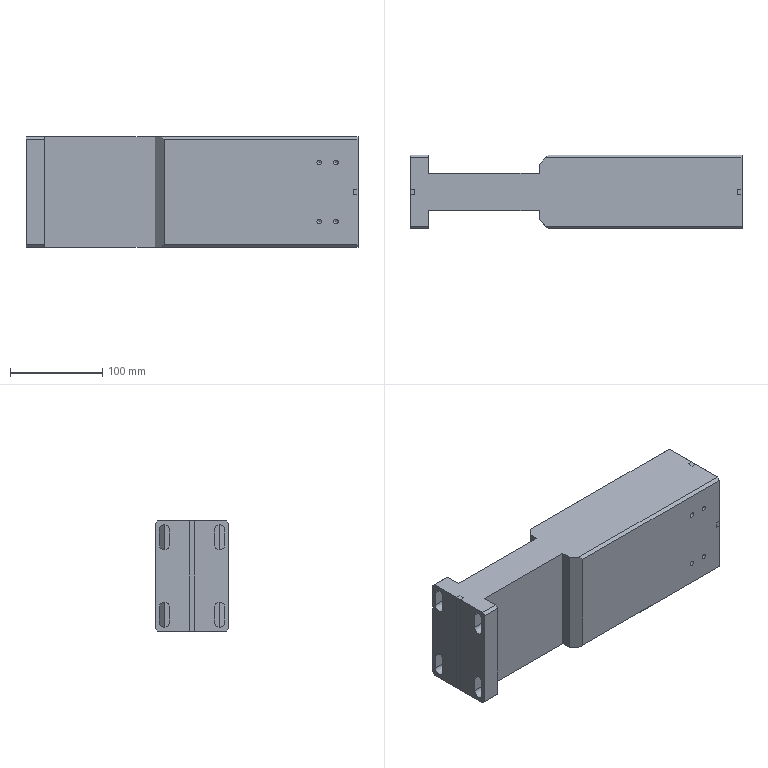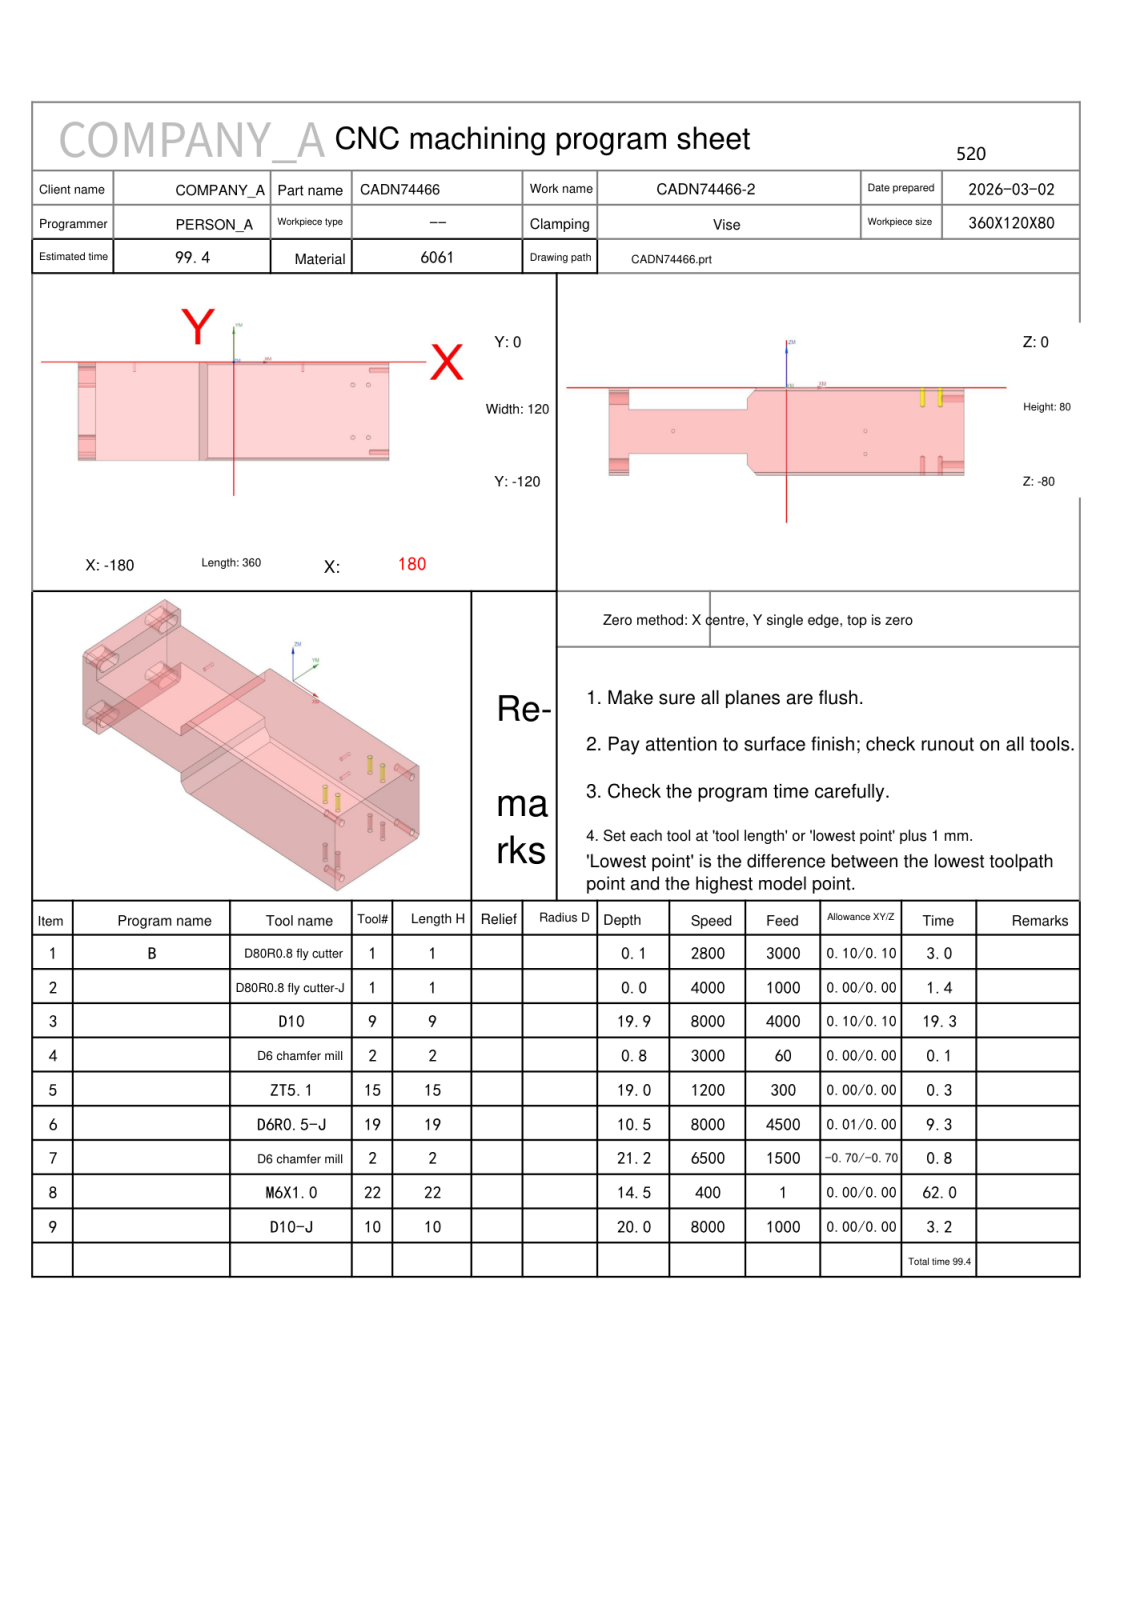NC program | NX | posted by the shop | part box 360 x 80 x 120 mm
Lines 4234 to 6245 of 6245:
N4 T02 M06
(D6 chamfer mill  D=6. R=0. H=02 ce=0.00 di=0.10)
G00 G90 G54 X138. Y-92. M03 S3000
G43 H02 Z50.
M08
G98 G81 X138. Y-92. Z-.8 R1. F60.
X156.
Y-28.
X138.
G80
G00 Z50.
G91 G28 Z0.0
M05
M09
G91 G28 Z0.0
M01
N5 T15 M06
(ZT5.1 D=5.1 DR_a=118 H=15)
G00 G90 G54 X138. Y-92. M03 S1200
G43 H15 Z50.
M08
G98 G83 X138. Y-92. Z-19. R1. F300. Q1.
X156.
Y-28.
X138.
G80
G00 Z50.
G91 G28 Z0.0
M05
M09
G91 G28 Z0.0
M01
N6 T19 M06
(D6R0.5-J  D=6. R=0.5 H=19 ce=0.01 di=0.00)
G00 G90 G54 X-32.786 Y-123.359 M03 S8000
G43 H19 Z14.5
M08
Z.429
G01 Z-.071 F4500.
Y-118.232
Y-1.768
X-32.857 Y-1.697 Z-.141
Y-118.303
X-32.927 Y-118.375 Z-.212
X-32.929 Y-118.275
Y-1.725
X-32.927 Y-1.625
X-32.996 Y-1.554 Z-.283
X-33. Y-1.725
Y-118.275
X-32.996 Y-118.446
X-33.068 Y-118.517 Z-.354
X-33.071 Y-118.275
Y-1.725
X-33.068 Y-1.483
X-33.14 Y-1.412 Z-.424
X-33.141 Y-2.722
Y-117.278
X-33.14 Y-118.588
X-33.21 Y-118.66 Z-.495
X-33.212 Y-118.622
Y-1.378
X-33.21 Y-1.34
X-33.28 Y-1.269 Z-.566
X-33.283 Y-1.378
Y-118.622
X-33.28 Y-118.731
X-33.35 Y-118.802 Z-.636
X-33.354 Y-118.622
Y-1.378
X-33.35 Y-1.198
X-33.421 Y-1.127 Z-.707
X-33.424 Y-1.378
Y-118.622
X-33.421 Y-118.873
X-33.494 Y-118.944 Z-.778
X-33.495 Y-117.631
Y-2.369
X-33.494 Y-1.056
X-33.563 Y-.985 Z-.849
X-33.566 Y-1.031
Y-118.969
X-33.563 Y-119.015
X-33.633 Y-119.085 Z-.919
X-33.636 Y-118.969
Y-1.031
X-33.633 Y-.915
X-33.704 Y-.844 Z-.99
X-33.707 Y-1.031
Y-118.969
X-33.704 Y-119.156
X-33.775 Y-119.227 Z-1.061
X-33.778 Y-118.969
Y-1.031
X-33.775 Y-.773
X-33.848 Y-.703 Z-1.131
Y-2.015
Y-117.985
Y-119.297
X-33.917 Y-119.368 Z-1.202
X-33.919 Y-119.316
Y-.684
X-33.917 Y-.632
X-33.987 Y-.562 Z-1.273
X-33.99 Y-.684
Y-119.316
X-33.987 Y-119.439
X-34.057 Y-119.509 Z-1.344
X-34.061 Y-119.316
Y-.684
X-34.057 Y-.491
X-34.129 Y-.42 Z-1.414
X-34.131 Y-1.732
Y-118.268
X-34.129 Y-119.58
X-34.202 Y-119.65 Z-1.485
Y-118.339
Y-1.661
Y-.35
X-34.27 Y-.279 Z-1.556
X-34.273 Y-.337
Y-119.663
X-34.27 Y-119.721
X-34.34 Y-119.791 Z-1.626
X-34.343 Y-119.663
Y-.337
X-34.34 Y-.208
X-34.411 Y-.138 Z-1.697
X-34.414 Y-.337
Y-119.663
X-34.411 Y-119.862
X-34.482 Y-119.932 Z-1.768
X-34.485 Y-118.621
Y-1.379
X-34.482 Y-.068
X-34.555 Y.002 Z-1.838
X-34.556 Y-1.308
Y-118.692
X-34.555 Y-120.002
X-34.624 Y-120.072 Z-1.909
X-34.626 Y-120.009
Y.009
X-34.624 Y.072
X-34.694 Y.142 Z-1.98
X-34.697 Y.009
Y-120.009
X-34.694 Y-120.142
X-34.764 Y-120.212 Z-2.051
X-34.768 Y-120.009
Y.009
X-34.764 Y.212
X-34.836 Y.282 Z-2.121
X-34.838 Y-1.025
Y-118.975
X-34.836 Y-120.282
X-34.909 Y-120.352 Z-2.192
Y-119.046
Y-.954
Y.352
X-34.977 Y.422 Z-2.263
X-34.98 Y.356
Y-120.356
X-34.977 Y-120.422
X-35.047 Y-120.492 Z-2.333
X-35.051 Y-120.356
Y.356
X-35.047 Y.492
X-35.118 Y.562 Z-2.404
X-35.121 Y.356
Y-120.356
X-35.118 Y-120.562
X-35.19 Y-120.632 Z-2.475
X-35.192 Y-119.328
Y-.672
X-35.19 Y.632
X-35.263 Y.703 Z-2.546
Y-.601
Y-119.399
Y-120.703
X-35.331 Y-120.772 Z-2.616
X-35.333 Y-120.703
Y.703
X-35.331 Y.772
X-35.401 Y.842 Z-2.687
X-35.404 Y.703
Y-120.703
X-35.401 Y-120.842
X-35.471 Y-120.912 Z-2.758
X-35.475 Y-120.703
Y.703
X-35.471 Y.912
X-35.543 Y.982 Z-2.828
X-35.546 Y-.318
Y-119.682
X-35.543 Y-120.982
X-35.616 Y-121.05 Z-2.899
Y-119.753
Y-.247
Y1.05
X-35.652 Y1.056 Z-2.934
X-35.686 Y1.061 Z-2.97
X-35.687 Y-.177
Y-119.823
X-35.686 Y-121.061
X-35.722 Y-121.062 Z-3.005
X-35.757 Z-3.041
X-35.758 Y-119.894
Y-.106
X-35.757 Y1.062
X-35.793 Y1.063 Z-3.076
X-35.828 Z-3.111
Y-.035
Y-119.965
Y-121.063
X-35.864 Z-3.147
X-35.898 Y-121.064 Z-3.182
X-35.899 Y-120.
Y0.0
X-35.898 Y1.064
X-35.934 Z-3.217
X-35.969 Y1.065 Z-3.253
X-35.97 Y0.0
Y-120.
X-35.969 Y-121.065
X-36.005 Z-3.288
X-36.04 Z-3.323
X-36.041 Y-120.
Y0.0
X-36.04 Y1.065
X-36.076 Y1.066 Z-3.359
X-36.11 Z-3.394
X-36.111 Y0.0
Y-120.
X-36.11 Y-121.066
X-36.147 Z-3.429
X-36.181 Y-121.067 Z-3.465
X-36.182 Y-120.
Y0.0
X-36.181 Y1.067
X-36.217 Z-3.5
X-36.252 Y1.068 Z-3.536
X-36.253 Y0.0
Y-120.
X-36.252 Y-121.067
X-36.288 Y-121.068 Z-3.571
X-36.322 Z-3.606
X-36.323 Y-120.
Y0.0
X-36.322 Y1.068
X-36.359 Y1.069 Z-3.642
X-36.393 Z-3.677
X-36.394 Y0.0
Y-120.
X-36.393 Y-121.069
X-36.429 Z-3.712
X-36.464 Y-121.07 Z-3.748
X-36.465 Y-120.
Y0.0
X-36.464 Y1.07
X-36.5 Z-3.783
X-36.534 Z-3.818
X-36.535 Y0.0
Y-120.
X-36.534 Y-121.07
X-36.571 Y-121.071 Z-3.854
X-36.605 Z-3.889
X-36.606 Y-120.
Y0.0
X-36.605 Y1.071
X-36.642 Y1.072 Z-3.924
X-36.676 Z-3.96
X-36.677 Y0.0
Y-120.
X-36.676 Y-121.072
X-36.712 Z-3.995
X-36.746 Y-121.073 Z-4.031
X-36.748 Y-120.
Y0.0
X-36.746 Y1.073
X-36.783 Z-4.066
X-36.817 Z-4.101
X-36.818 Y0.0
Y-120.
X-36.817 Y-121.073
X-36.854 Y-121.074 Z-4.137
X-36.888 Z-4.172
X-36.889 Y-120.
Y0.0
X-36.888 Y1.074
X-36.924 Y1.075 Z-4.207
X-36.958 Z-4.243
X-36.96 Y1.05
Y-121.05
X-36.958 Y-121.075
X-36.995 Z-4.278
X-37.029 Y-121.076 Z-4.313
X-37.03 Y-121.05
Y1.05
X-37.029 Y1.076
X-37.066 Z-4.349
X-37.1 Z-4.384
X-37.101 Y1.05
Y-121.05
X-37.1 Y-121.076
X-37.137 Y-121.077 Z-4.419
X-37.17 Z-4.455
X-37.172 Y-121.05
Y1.05
X-37.17 Y1.077
X-37.207 Z-4.49
X-37.241 Y1.078 Z-4.525
X-37.243 Y1.05
Y-121.05
X-37.241 Y-121.078
X-37.278 Z-4.561
X-37.312 Z-4.596
X-37.313 Y-121.05
Y1.05
X-37.312 Y1.078
X-37.349 Y1.079 Z-4.632
X-37.383 Z-4.667
X-37.384 Y1.05
Y-121.05
X-37.383 Y-121.079
X-37.419 Z-4.702
X-37.453 Z-4.738
X-37.455 Y-121.05
Y1.05
X-37.453 Y1.079
X-37.49 Y1.08 Z-4.773
X-37.524 Z-4.808
X-37.525 Y1.05
Y-121.05
X-37.524 Y-121.08
X-37.561 Z-4.844
X-37.595 Z-4.879
X-37.596 Y-121.05
Y1.05
X-37.595 Y1.08
X-37.632 Y1.081 Z-4.914
X-37.665 Z-4.95
X-37.667 Y1.05
Y-121.05
X-37.665 Y-121.081
X-37.702 Z-4.985
X-37.736 Z-5.02
X-37.738 Y-121.05
Y1.05
X-37.736 Y1.081
X-37.773 Y1.082 Z-5.056
X-37.807 Z-5.091
X-37.808 Y1.05
Y-121.05
X-37.807 Y-121.082
X-37.844 Z-5.127
X-37.877 Z-5.162
X-37.879 Y-121.05
Y1.05
X-37.877 Y1.082
X-37.914 Y1.083 Z-5.197
X-37.948 Z-5.233
X-37.95 Y1.05
Y-121.05
X-37.948 Y-121.083
X-37.985 Z-5.268
X-38.019 Z-5.303
X-38.02 Y-121.05
Y1.05
X-38.019 Y1.083
X-38.056 Y1.084 Z-5.339
X-38.089 Z-5.374
X-38.091 Y1.05
Y-121.05
X-38.089 Y-121.084
X-38.126 Z-5.409
X-38.16 Z-5.445
X-38.162 Y-121.05
Y1.05
X-38.16 Y1.084
X-38.197 Z-5.48
X-38.231 Y1.085 Z-5.515
X-38.233 Y1.05
Y-121.05
X-38.231 Y-121.085
X-38.268 Z-5.551
X-38.302 Z-5.586
X-38.303 Y-121.05
Y1.05
X-38.302 Y1.085
X-38.339 Z-5.622
X-38.372 Y1.086 Z-5.657
X-38.374 Y1.05
Y-121.05
X-38.372 Y-121.086
X-38.409 Z-5.692
X-38.443 Z-5.728
X-38.445 Y-121.05
Y1.05
X-38.443 Y1.086
X-38.48 Z-5.763
X-38.514 Y1.087 Z-5.798
X-38.515 Y1.05
Y-121.05
X-38.514 Y-121.087
X-38.551 Z-5.834
X-38.584 Z-5.869
X-38.586 Y-121.05
Y1.05
X-38.584 Y1.087
X-38.621 Z-5.904
X-38.655 Z-5.94
X-38.657 Y1.05
Y-121.05
X-38.655 Y-121.087
X-38.692 Z-5.975
X-38.726 Z-6.01
X-38.728 Y-120.
Y1.05
X-38.726 Y1.088
X-38.763 Z-6.046
X-38.796 Z-6.081
X-38.798 Y1.05
Y-121.05
X-38.796 Y-121.088
X-38.834 Z-6.116
X-38.867 Z-6.152
X-38.869 Y-121.05
Y1.05
X-38.867 Y1.088
X-38.904 Z-6.187
X-38.938 Z-6.223
X-38.94 Y1.05
Y-121.05
X-38.938 Y-121.088
X-38.975 Z-6.258
X-39.009 Z-6.293
X-39.01 Y-121.05
Y1.05
X-39.009 Y1.088
X-39.046 Z-6.329
X-39.079 Z-6.364
X-39.081 Y1.05
Y-121.05
X-39.079 Y-121.088
X-39.116 Z-6.399
X-39.152 Z-6.435
Y-120.
Y0.0
Y1.088
X-39.187 Z-6.47
X-39.221 Z-6.505
X-39.222 Y1.05
Y-121.05
X-39.221 Y-121.088
X-39.258 Z-6.541
X-39.291 Y-121.089 Z-6.576
X-39.293 Y-121.05
Y1.05
X-39.291 Y1.088
X-39.329 Z-6.611
X-39.362 Y1.089 Z-6.647
X-39.364 Y1.05
Y-121.05
X-39.362 Y-121.089
X-39.399 Z-6.682
X-39.433 Z-6.718
X-39.435 Y-121.05
Y1.05
X-39.433 Y1.089
X-39.47 Z-6.753
X-39.504 Z-6.788
X-39.505 Y1.05
Y-121.05
X-39.504 Y-121.089
X-39.541 Z-6.824
X-39.574 Z-6.859
X-39.576 Y-121.05
Y1.05
X-39.574 Y1.089
X-39.611 Z-6.894
X-39.645 Z-6.93
X-39.647 Y1.05
Y-121.05
X-39.645 Y-121.089
X-39.682 Z-6.965
X-39.716 Z-7.
X-39.717 Y-121.05
Y1.05
X-39.716 Y1.089
X-39.753 Z-7.036
X-39.786 Z-7.071
X-39.788 Y1.05
Y-121.05
X-39.786 Y-121.089
X-39.824 Z-7.106
X-39.857 Z-7.142
X-39.859 Y-121.05
Y1.05
X-39.857 Y1.089
X-39.894 Z-7.177
X-39.928 Z-7.212
X-39.93 Y1.05
Y-121.05
X-39.928 Y-121.089
X-39.965 Z-7.248
X-39.998 Z-7.283
X-40. Y-121.05
Y1.05
X-39.998 Y1.089
X-40.036 Z-7.319
X-40.069 Z-7.354
X-40.071 Y1.05
Y-121.05
X-40.069 Y-121.089
X-40.106 Z-7.389
X-40.14 Z-7.425
X-40.142 Y-121.05
Y1.05
X-40.14 Y1.089
X-40.177 Z-7.46
X-40.211 Z-7.495
X-40.212 Y1.05
Y-121.05
X-40.211 Y-121.089
X-40.248 Z-7.531
X-40.281 Z-7.566
X-40.283 Y-121.05
Y1.05
X-40.281 Y1.089
X-40.319 Z-7.601
X-40.352 Y1.088 Z-7.637
X-40.354 Y1.05
Y-121.05
X-40.352 Y-121.088
X-40.389 Z-7.672
X-40.423 Z-7.707
X-40.425 Y-121.05
Y1.05
X-40.423 Y1.088
X-40.46 Z-7.743
X-40.493 Z-7.778
X-40.495 Y1.05
Y-121.05
X-40.493 Y-121.088
X-40.531 Z-7.814
X-40.564 Z-7.849
X-40.566 Y-121.05
Y1.05
X-40.564 Y1.088
X-40.601 Z-7.884
X-40.635 Y1.087 Z-7.92
X-40.637 Y1.05
Y-121.05
X-40.635 Y-121.087
X-40.672 Z-7.955
X-40.706 Z-7.99
X-40.707 Y-121.05
Y1.05
X-40.706 Y1.087
X-40.743 Z-8.026
X-40.776 Z-8.061
X-40.778 Y1.05
Y-121.05
X-40.776 Y-121.087
X-40.813 Z-8.096
X-40.847 Y-121.086 Z-8.132
X-40.849 Y-121.05
Y1.05
X-40.847 Y1.087
X-40.884 Z-8.167
X-40.918 Y1.086 Z-8.202
X-40.92 Y1.05
Y-121.05
X-40.918 Y-121.086
X-40.955 Z-8.238
X-40.989 Z-8.273
X-40.99 Y-121.05
Y1.05
X-40.989 Y1.086
X-41.026 Z-8.309
X-41.059 Z-8.344
X-41.061 Y1.05
Y-121.05
X-41.059 Y-121.086
X-41.096 Z-8.379
X-41.13 Z-8.415
X-41.132 Y-121.05
Y1.05
X-41.13 Y1.086
X-41.167 Y1.085 Z-8.45
X-41.201 Z-8.485
X-41.202 Y1.05
Y-121.05
X-41.201 Y-121.085
X-41.238 Z-8.521
X-41.271 Z-8.556
X-41.273 Y-121.05
Y1.05
X-41.271 Y1.085
X-41.308 Z-8.591
X-41.342 Z-8.627
X-41.344 Y1.05
Y-121.05
X-41.342 Y-121.085
X-41.379 Z-8.662
X-41.413 Y-121.084 Z-8.697
X-41.415 Y-121.05
Y1.05
X-41.413 Y1.084
X-41.45 Z-8.733
X-41.484 Z-8.768
X-41.485 Y1.05
Y-121.05
X-41.484 Y-121.084
X-41.521 Z-8.803
X-41.554 Z-8.839
X-41.556 Y-121.05
Y1.05
X-41.554 Y1.084
X-41.591 Y1.083 Z-8.874
X-41.625 Z-8.91
X-41.627 Y1.05
Y-121.05
X-41.625 Y-121.083
X-41.662 Z-8.945
X-41.696 Z-8.98
X-41.697 Y-121.05
Y1.05
X-41.696 Y1.083
X-41.733 Y1.082 Z-9.016
X-41.766 Z-9.051
X-41.768 Y1.05
Y-121.05
X-41.766 Y-121.082
X-41.803 Z-9.086
X-41.837 Z-9.122
X-41.839 Y-121.05
Y1.05
X-41.837 Y1.082
X-41.874 Z-9.157
X-41.908 Y1.081 Z-9.192
X-41.909 Y1.05
Y-121.05
X-41.908 Y-121.081
X-41.945 Z-9.228
X-41.979 Z-9.263
X-41.98 Y-121.05
Y1.05
X-41.979 Y1.081
X-42.016 Z-9.298
X-42.049 Y1.08 Z-9.334
X-42.051 Y1.05
Y-121.05
X-42.049 Y-121.08
X-42.086 Z-9.369
X-42.12 Z-9.405
X-42.122 Y-121.05
Y1.05
X-42.12 Y1.08
X-42.157 Z-9.44
X-42.191 Y1.079 Z-9.475
X-42.192 Y1.05
Y-121.05
X-42.191 Y-121.079
X-42.228 Z-9.511
X-42.262 Z-9.546
X-42.263 Y-121.05
Y1.05
X-42.262 Y1.079
X-42.298 Z-9.581
X-42.332 Y1.078 Z-9.617
X-42.334 Y1.05
Y-121.05
X-42.332 Y-121.078
X-42.369 Z-9.652
X-42.403 Z-9.687
X-42.404 Y-121.05
Y1.05
X-42.403 Y1.078
X-42.44 Z-9.723
X-42.474 Z-9.758
X-42.475 Y1.05
Y-121.05
X-42.474 Y-121.077
X-42.511 Z-9.793
X-42.545 Z-9.829
X-42.546 Y-121.05
Y1.05
X-42.544 Y1.077
X-42.581 Z-9.864
X-42.616 Z-9.899
X-42.617 Y0.0
Y-120.
X-42.616 Y-121.077
X-42.652 Y-121.076 Z-9.935
X-42.686 Z-9.97
X-42.687 Y-121.05
Y1.05
X-42.686 Y1.076
X-42.723 Z-10.006
X-42.757 Z-10.041
X-42.758 Y1.05
Y-121.05
X-42.757 Y-121.076
X-42.793 Y-121.075 Z-10.076
X-42.827 Z-10.112
X-42.829 Y-121.05
Y1.05
X-42.827 Y1.075
X-42.864 Z-10.147
X-42.898 Z-10.182
Y-121.075
X-42.935 Y-121.074 Z-10.218
X-42.969 Z-10.253
Y1.074
X-43.001 Z-10.284
X-43.031 Z-10.315
Y-121.074
X-43.063 Z-10.346
X-43.092 Y-121.073 Z-10.377
Y1.073
X-43.125 Z-10.407
X-43.154 Z-10.438
Y-121.073
X-43.186 Z-10.469
X-43.216 Z-10.5
Y1.073
G00 Z14.5
G00 G90 X-153.773 Y-119.784 M03 S8000
Z14.5
Z.429
G01 Z-.071 F4500.
X-158.926 Y-119.785
X-181.074 Y-119.788
Y-119.823 Z-.106
Y-119.858 Z-.141
X-158.926 Y-119.856
Y-119.894 Z-.177
Y-119.926 Z-.212
X-159.074 Y-119.929
X-180.
X-181.074
X-181.075 Y-119.965 Z-.247
Y-120. Z-.283
X-180.
X-159.074
X-158.925 Y-119.997
Y-120.035 Z-.318
Y-120.068 Z-.354
X-159.074 Y-120.071
X-180.
X-181.075
Y-120.106 Z-.389
X-181.076 Y-120.141 Z-.424
X-180.
X-159.074
X-158.925 Y-120.138
X-158.924 Y-120.177 Z-.46
Y-120.209 Z-.495
X-159.074 Y-120.212
X-180.
X-181.076
Y-120.247 Z-.53
Y-120.283 Z-.566
X-180.
X-159.074
X-158.924 Y-120.28
Y-120.318 Z-.601
X-158.923 Y-120.351 Z-.636
X-159.074 Y-120.354
X-180.
X-181.077 Y-120.353
Y-120.389 Z-.672
Y-120.424 Z-.707
X-180.
X-159.074
X-158.923 Y-120.421
Y-120.46 Z-.742
Y-120.492 Z-.778
X-159.074 Y-120.495
X-180.
X-181.077
X-181.078 Y-120.53 Z-.813
Y-120.566 Z-.849
X-180.
X-159.074
X-158.922 Y-120.563
Y-120.601 Z-.884
Y-120.634 Z-.919
X-159.074 Y-120.636
X-180.
X-181.078
Y-120.672 Z-.955
Y-120.707 Z-.99
X-180.
X-159.074
X-158.922 Y-120.704
X-158.921 Y-120.742 Z-1.025
Y-120.775 Z-1.061
X-159.074 Y-120.778
X-180.
X-181.079
Y-120.813 Z-1.096
Y-120.848 Z-1.131
X-180.
X-159.074
X-158.921 Y-120.846
Y-120.884 Z-1.167
Y-120.916 Z-1.202
X-159.074 Y-120.919
X-180.
X-181.079
Y-120.955 Z-1.237
Y-120.99 Z-1.273
X-180.
X-159.074
X-158.921 Y-120.987
Y-121.025 Z-1.308
Y-121.058 Z-1.344
X-159.074 Y-121.061
X-180.
X-181.079
Y-121.096 Z-1.379
Y-121.131 Z-1.414
X-180.
X-160.
X-158.921
Y-121.167 Z-1.45
Y-121.199 Z-1.485
X-159.074 Y-121.202
X-180.
X-181.079
Y-121.237 Z-1.52
Y-121.273 Z-1.556
X-180.
X-159.074
X-158.921 Y-121.27
Y-121.308 Z-1.591
Y-121.341 Z-1.626
X-159.074 Y-121.343
X-180.
X-181.079
Y-121.379 Z-1.662
Y-121.414 Z-1.697
X-180.
X-159.074
X-158.921 Y-121.411
Y-121.45 Z-1.732
Y-121.482 Z-1.768
X-159.074 Y-121.485
X-180.
X-181.079
Y-121.52 Z-1.803
Y-121.556 Z-1.838
X-180.
X-159.074
X-158.921 Y-121.553
Y-121.591 Z-1.874
Y-121.623 Z-1.909
X-159.074 Y-121.626
X-180.
X-181.079
Y-121.662 Z-1.945
Y-121.697 Z-1.98
X-180.
X-159.074
X-158.921 Y-121.694
Y-121.732 Z-2.015
Y-121.765 Z-2.051
X-159.074 Y-121.768
X-180.
X-181.079
Y-121.803 Z-2.086
Y-121.838 Z-2.121
X-180.
X-159.074
X-158.921 Y-121.836
Y-121.874 Z-2.157
Y-121.906 Z-2.192
X-159.074 Y-121.909
X-180.
X-181.079
Y-121.944 Z-2.227
Y-121.98 Z-2.263
X-180.
X-159.074
X-158.922 Y-121.977
Y-122.015 Z-2.298
Y-122.048 Z-2.333
X-159.074 Y-122.051
X-180.
X-181.078
Y-122.086 Z-2.369
Y-122.121 Z-2.404
X-180.
X-159.074
X-158.922 Y-122.118
Y-122.157 Z-2.44
Y-122.189 Z-2.475
X-159.074 Y-122.192
X-180.
X-181.078
X-181.077 Y-122.227 Z-2.51
Y-122.263 Z-2.546
X-180.
X-159.074
X-158.923 Y-122.26
Y-122.298 Z-2.581
Y-122.331 Z-2.616
X-159.074 Y-122.333
X-180.
X-181.077
Y-122.369 Z-2.652
X-181.076 Y-122.404 Z-2.687
X-180.
X-159.074
X-158.924 Y-122.401
Y-122.439 Z-2.722
Y-122.472 Z-2.758
X-159.074 Y-122.475
X-180.
X-181.076
Y-122.51 Z-2.793
Y-122.546 Z-2.828
X-180.
X-159.074
X-158.924 Y-122.543
X-158.925 Y-122.581 Z-2.864
Y-122.613 Z-2.899
X-159.074 Y-122.616
X-180.
X-181.075
Y-122.652 Z-2.934
Y-122.687 Z-2.97
X-180.
X-159.074
X-158.925 Y-122.684
Y-122.722 Z-3.005
Y-122.755 Z-3.041
X-159.074 Y-122.758
X-180.
X-181.075
X-181.074 Y-122.793 Z-3.076
Y-122.828 Z-3.111
X-180.
X-159.074
X-158.926 Y-122.825
Y-122.864 Z-3.147
Y-122.896 Z-3.182
X-181.074 Y-122.899
Y-122.934 Z-3.217
X-181.073 Y-122.97 Z-3.253
X-158.927 Y-122.967
Y-123.001 Z-3.284
Y-123.029 Z-3.315
X-181.073 Y-123.032
Y-123.063 Z-3.345
Y-123.093 Z-3.376
X-158.927 Y-123.091
Y-123.124 Z-3.407
X-158.928 Y-123.152 Z-3.438
X-181.073 Y-123.155
X-181.072 Y-123.186 Z-3.469
Y-123.217 Z-3.5
X-158.928 Y-123.214
G00 Z14.5
X-186.221 Y-.212
Z.429
G01 Z-.071
X-181.074
X-158.926 Y-.215
Y-.177 Z-.106
Y-.144 Z-.141
X-181.074 Y-.142
Y-.106 Z-.177
Y-.071 Z-.212
X-180.
X-159.074
X-158.926 Y-.074
X-158.925 Y-.035 Z-.247
Y-.003 Z-.283
X-159.074 Y0.0
X-180.
X-181.075
Y.035 Z-.318
Y.071 Z-.354
X-180.
X-159.074
X-158.925 Y.068
Y.106 Z-.389
Y.138 Z-.424
X-159.074 Y.141
X-180.
X-181.076
Y.177 Z-.46
Y.212 Z-.495
X-180.
X-159.074
X-158.924 Y.209
Y.247 Z-.53
Y.28 Z-.566
X-159.074 Y.283
X-180.
X-181.076
Y.318 Z-.601
X-181.077 Y.353 Z-.636
X-180. Y.354
X-159.074
X-158.923 Y.351
Y.389 Z-.672
Y.421 Z-.707
X-159.074 Y.424
X-180.
X-181.077
Y.46 Z-.742
Y.495 Z-.778
X-180.
X-159.074
X-158.923 Y.492
X-158.922 Y.53 Z-.813
Y.563 Z-.849
X-159.074 Y.566
X-180.
X-181.078
Y.601 Z-.884
Y.636 Z-.919
X-180.
X-159.074
X-158.922 Y.634
Y.672 Z-.955
Y.704 Z-.99
X-159.074 Y.707
X-180.
X-181.078
X-181.079 Y.742 Z-1.025
Y.778 Z-1.061
X-180.
X-159.074
X-158.921 Y.775
Y.813 Z-1.096
Y.846 Z-1.131
X-159.074 Y.848
X-180.
X-181.079
Y.884 Z-1.167
Y.919 Z-1.202
X-180.
X-159.074
X-158.921 Y.916
Y.955 Z-1.237
Y.987 Z-1.273
X-159.074 Y.99
X-180.
X-181.079
Y1.025 Z-1.308
Y1.061 Z-1.344
X-180.
X-159.074
X-158.921 Y1.058
Y1.096 Z-1.379
Y1.131 Z-1.414
X-160.
X-180.
X-181.079
Y1.167 Z-1.45
Y1.202 Z-1.485
X-180.
X-159.074
X-158.921 Y1.199
Y1.237 Z-1.52
Y1.27 Z-1.556
X-159.074 Y1.273
X-180.
X-181.079
Y1.308 Z-1.591
Y1.343 Z-1.626
X-180.
X-159.074
X-158.921 Y1.341
Y1.379 Z-1.662
Y1.411 Z-1.697
X-159.074 Y1.414
X-180.
X-181.079
Y1.45 Z-1.732
Y1.485 Z-1.768
X-180.
X-159.074
X-158.921 Y1.482
Y1.52 Z-1.803
Y1.553 Z-1.838
X-159.074 Y1.556
X-180.
X-181.079
Y1.591 Z-1.874
Y1.626 Z-1.909
X-180.
X-159.074
X-158.921 Y1.623
Y1.662 Z-1.945
Y1.694 Z-1.98
X-159.074 Y1.697
X-180.
X-181.079
Y1.732 Z-2.015
Y1.768 Z-2.051
X-180.
X-159.074
X-158.921 Y1.765
Y1.803 Z-2.086
Y1.836 Z-2.121
X-159.074 Y1.838
X-180.
X-181.079
Y1.874 Z-2.157
Y1.909 Z-2.192
X-180.
X-159.074
X-158.921 Y1.906
Y1.944 Z-2.227
X-158.922 Y1.977 Z-2.263
X-159.074 Y1.98
X-180.
X-181.079
X-181.078 Y2.015 Z-2.298
Y2.051 Z-2.333
X-180.
X-159.074
X-158.922 Y2.048
Y2.086 Z-2.369
Y2.118 Z-2.404
X-159.074 Y2.121
X-180.
X-181.078
Y2.157 Z-2.44
Y2.192 Z-2.475
X-180.
X-159.074
X-158.922 Y2.189
X-158.923 Y2.227 Z-2.51
Y2.26 Z-2.546
X-159.074 Y2.263
X-180.
X-181.077
Y2.298 Z-2.581
Y2.333 Z-2.616
X-180.
X-159.074
X-158.923 Y2.331
Y2.369 Z-2.652
X-158.924 Y2.401 Z-2.687
X-159.074 Y2.404
X-180.
X-181.076
Y2.439 Z-2.722
Y2.475 Z-2.758
X-180.
X-159.074
X-158.924 Y2.472
Y2.51 Z-2.793
Y2.543 Z-2.828
X-159.074 Y2.546
X-180.
X-181.076
X-181.075 Y2.581 Z-2.864
Y2.616 Z-2.899
X-180.
X-159.074
X-158.925 Y2.613
Y2.652 Z-2.934
Y2.684 Z-2.97
X-159.074 Y2.687
X-180.
X-181.075
Y2.722 Z-3.005
Y2.758 Z-3.041
X-180.
X-159.074
X-158.925 Y2.755
X-158.926 Y2.793 Z-3.076
Y2.825 Z-3.111
X-159.074 Y2.828
X-180.
X-181.074
Y2.864 Z-3.147
Y2.899 Z-3.182
X-158.926 Y2.896
Y2.934 Z-3.217
X-158.927 Y2.967 Z-3.253
X-181.073 Y2.97
Y3.001 Z-3.284
Y3.032 Z-3.315
X-158.927 Y3.029
Y3.063 Z-3.345
Y3.091 Z-3.376
X-181.073 Y3.093
Y3.124 Z-3.407
Y3.155 Z-3.438
X-158.928 Y3.152
Y3.186 Z-3.469
Y3.214 Z-3.5
X-181.072 Y3.217
G00 Z14.5
X-36.361 Y-.215
Z.429
G01 Z-.071
X-31.233
X181.074 Y-.213
Y-.177 Z-.106
Y-.143 Z-.141
X-31.304 Y-.145
X-31.376 Y-.073 Z-.212
X-30.066 Y-.071
X180.
X181.074 Y-.072
X181.075 Y-.035 Z-.247
Y-.001 Z-.283
X180. Y0.0
X-30.136
X-31.447
X-31.518 Y.068 Z-.354
X-31.447 Y.071
X180.
X181.075 Y.069
Y.106 Z-.389
Y.14 Z-.424
X180. Y.141
X-31.447
X-31.59 Y.138
X-31.661 Y.209 Z-.495
X-31.447 Y.212
X180.
X181.076 Y.211
Y.247 Z-.53
Y.282 Z-.566
X180. Y.283
X-30.419
X-31.733 Y.281
X-31.804 Y.353 Z-.636
X-30.49 Y.354
X180.
X181.076 Y.352
X181.077 Y.389 Z-.672
Y.423 Z-.707
X180. Y.424
X-31.793
X-31.875 Y.421
X-31.946 Y.492 Z-.778
X-31.793 Y.495
X180.
X181.077 Y.494
Y.53 Z-.813
X181.078 Y.564 Z-.849
X180. Y.566
X-31.793
X-32.017 Y.563
X-32.088 Y.635 Z-.919
X-30.773 Y.636
X181.053
X181.078 Y.635
Y.672 Z-.955
Y.706 Z-.99
X181.053 Y.707
X-30.844
X-32.158 Y.706
X-32.229 Y.775 Z-1.061
X-32.14 Y.778
X181.053
X181.079 Y.776
Y.813 Z-1.096
Y.847 Z-1.131
X181.053 Y.848
X-32.14
X-32.3 Y.845
X-32.371 Y.916 Z-1.202
X-32.14 Y.919
X181.053
X181.079 Y.918
Y.955 Z-1.237
Y.989 Z-1.273
X181.053 Y.99
X-31.126
X-32.442 Y.988
X-32.512 Y1.059 Z-1.344
X-32.487 Y1.061
X181.053
X181.079 Y1.059
Y1.096 Z-1.379
Y1.131 Z-1.414
X180.
X-31.268
X-32.583
X-32.654 Y1.199 Z-1.485
X-32.487 Y1.202
X181.053
X181.079 Y1.201
Y1.237 Z-1.52
Y1.271 Z-1.556
X181.053 Y1.273
X-32.487
X-32.725 Y1.27
X-32.796 Y1.342 Z-1.626
X-31.48 Y1.343
X181.053
X181.079 Y1.342
Y1.379 Z-1.662
Y1.413 Z-1.697
X181.053 Y1.414
X-32.833
X-32.866 Y1.412
X-32.937 Y1.482 Z-1.768
X-32.833 Y1.485
X181.053
X181.079 Y1.484
Y1.52 Z-1.803
Y1.554 Z-1.838
X181.053 Y1.556
X-32.833
X-33.007 Y1.552
X-33.077 Y1.623 Z-1.909
X-32.833 Y1.626
X181.053
X181.079 Y1.625
Y1.662 Z-1.945
Y1.696 Z-1.98
X181.053 Y1.697
X-31.833
X-33.147 Y1.696
X-33.217 Y1.766 Z-2.051
X-33.18 Y1.768
X181.053
X181.079 Y1.766
Y1.803 Z-2.086
Y1.837 Z-2.121
X181.053 Y1.838
X-33.18
X-33.288 Y1.835
X-33.358 Y1.906 Z-2.192
X-33.18 Y1.909
X181.053
X181.079 Y1.908
Y1.944 Z-2.227
X181.078 Y1.979 Z-2.263
X181.053 Y1.98
X-33.18
X-33.428 Y1.977
X-33.498 Y2.049 Z-2.333
X-32.187 Y2.051
X181.053
X181.078 Y2.049
Y2.086 Z-2.369
Y2.12 Z-2.404
X181.053 Y2.121
X-33.527
X-33.569 Y2.119
X-33.639 Y2.189 Z-2.475
X-33.527 Y2.192
X180.
X181.077 Y2.191
Y2.227 Z-2.51
Y2.261 Z-2.546
X180. Y2.263
X-33.527
X-33.709 Y2.259
X-33.779 Y2.33 Z-2.616
X-33.527 Y2.333
X180.
X181.077 Y2.332
Y2.369 Z-2.652
X181.076 Y2.403 Z-2.687
X180. Y2.404
X-32.541
X-33.85 Y2.403
X-33.92 Y2.473 Z-2.758
X-33.873 Y2.475
X180.
X181.076 Y2.474
Y2.51 Z-2.793
Y2.544 Z-2.828
X180. Y2.546
X-33.873
X-33.99 Y2.542
X-34.06 Y2.612 Z-2.899
X-33.873 Y2.616
X180.
X181.075 Y2.615
Y2.652 Z-2.934
Y2.686 Z-2.97
X180. Y2.687
X-33.873
X-34.13 Y2.684
X-34.201 Y2.757 Z-3.041
X-32.894 Y2.758
X180.
X181.075 Y2.757
X181.074 Y2.793 Z-3.076
Y2.827 Z-3.111
X180. Y2.828
X-34.22
X-34.271 Y2.826
X-34.246 Y2.898 Z-3.182
X181.074
Y2.934 Z-3.217
X181.073 Y2.969 Z-3.253
X-34.198
X-34.136 Y3.029 Z-3.315
X181.073 Y3.031
Y3.063 Z-3.345
Y3.092 Z-3.376
X-34.075 Y3.09
X-34.013 Y3.152 Z-3.438
X181.072 Y3.154
Y3.186 Z-3.469
Y3.216 Z-3.5
X-33.951 Y3.214
G00 Z14.5
X186.223 Y-119.787
Z.429
G01 Z-.071
X181.074
X-31.233 Y-119.785
X-31.304 Y-119.855 Z-.141
X181.074 Y-119.857
Y-119.894 Z-.177
Y-119.928 Z-.212
X180. Y-119.929
X-30.066
X-31.376 Y-119.927
X-31.447 Y-120. Z-.283
X-30.136
X180.
X181.075 Y-119.999
Y-120.035 Z-.318
Y-120.069 Z-.354
X180. Y-120.071
X-31.447
X-31.518 Y-120.068
X-31.59 Y-120.138 Z-.424
X-31.447 Y-120.141
X180.
X181.075 Y-120.14
X181.076 Y-120.177 Z-.46
Y-120.211 Z-.495
X180. Y-120.212
X-31.447
X-31.661 Y-120.209
X-31.733 Y-120.281 Z-.566
X-30.419 Y-120.283
X180.
X181.076 Y-120.282
Y-120.318 Z-.601
Y-120.352 Z-.636
X180. Y-120.354
X-30.49
X-31.804 Y-120.353
X-31.875 Y-120.421 Z-.707
X-31.793 Y-120.424
X180.
X181.077 Y-120.423
Y-120.46 Z-.742
Y-120.494 Z-.778
X180. Y-120.495
X-31.793
X-31.946 Y-120.492
X-32.017 Y-120.563 Z-.849
X-31.793 Y-120.566
X180.
X181.078 Y-120.564
Y-120.601 Z-.884
Y-120.635 Z-.919
X181.053 Y-120.636
X-30.773
X-32.088 Y-120.635
X-32.158 Y-120.706 Z-.99
X-30.844 Y-120.707
X181.053
X181.078 Y-120.706
X181.079 Y-120.742 Z-1.025
Y-120.776 Z-1.061
X181.053 Y-120.778
X-32.14
X-32.229 Y-120.775
X-32.3 Y-120.845 Z-1.131
X-32.14 Y-120.848
X181.053
X181.079 Y-120.847
Y-120.884 Z-1.167
Y-120.918 Z-1.202
X181.053 Y-120.919
X-32.14
X-32.371 Y-120.916
X-32.442 Y-120.988 Z-1.273
X-31.126 Y-120.99
X181.053
X181.079 Y-120.989
Y-121.025 Z-1.308
Y-121.059 Z-1.344
X181.053 Y-121.061
X-32.487
X-32.512 Y-121.059
X-32.583 Y-121.131 Z-1.414
X-31.268
X180.94
X181.08 Y-121.13
Y-121.167 Z-1.45
X181.079 Y-121.201 Z-1.485
X181.053 Y-121.202
X-32.487
X-32.654 Y-121.199
X-32.725 Y-121.27 Z-1.556
X-32.487 Y-121.273
X181.053
X181.079 Y-121.271
Y-121.308 Z-1.591
Y-121.342 Z-1.626
X181.053 Y-121.343
X-31.48
X-32.796 Y-121.342
X-32.866 Y-121.412 Z-1.697
X-32.833 Y-121.414
X181.053
X181.079 Y-121.413
Y-121.45 Z-1.732
Y-121.484 Z-1.768
X181.053 Y-121.485
X-32.833
X-32.937 Y-121.482
X-33.007 Y-121.552 Z-1.838
X-32.833 Y-121.556
X181.053
X181.079 Y-121.554
Y-121.591 Z-1.874
Y-121.625 Z-1.909
X181.053 Y-121.626
X-32.833
X-33.077 Y-121.623
X-33.147 Y-121.696 Z-1.98
X-31.833 Y-121.697
X181.053
X181.079 Y-121.696
Y-121.732 Z-2.015
Y-121.766 Z-2.051
X181.053 Y-121.768
X-33.18
X-33.217 Y-121.766
X-33.288 Y-121.835 Z-2.121
X-33.18 Y-121.838
X181.053
X181.079 Y-121.837
Y-121.874 Z-2.157
Y-121.908 Z-2.192
X181.053 Y-121.909
X-33.18
X-33.358 Y-121.906
X-33.428 Y-121.977 Z-2.263
X-33.18 Y-121.98
X181.053
X181.078 Y-121.979
Y-122.015 Z-2.298
Y-122.049 Z-2.333
X181.053 Y-122.051
X-32.187
X-33.498 Y-122.049
X-33.569 Y-122.119 Z-2.404
X-33.527 Y-122.121
X181.053
X181.078 Y-122.12
Y-122.157 Z-2.44
X181.077 Y-122.191 Z-2.475
X180. Y-122.192
X-33.527
X-33.639 Y-122.189
X-33.709 Y-122.259 Z-2.546
X-33.527 Y-122.263
X180.
X181.077 Y-122.261
Y-122.298 Z-2.581
Y-122.332 Z-2.616
X180. Y-122.333
X-33.527
X-33.779 Y-122.33
X-33.85 Y-122.403 Z-2.687
X-32.541 Y-122.404
X180.
X181.076 Y-122.403
Y-122.439 Z-2.722
Y-122.474 Z-2.758
X180. Y-122.475
X-33.873
X-33.92 Y-122.473
X-33.99 Y-122.542 Z-2.828
X-33.873 Y-122.546
X180.
X181.076 Y-122.544
X181.075 Y-122.581 Z-2.864
Y-122.615 Z-2.899
X180. Y-122.616
X-33.873
X-34.06 Y-122.612
X-34.13 Y-122.684 Z-2.97
X-33.873 Y-122.687
X180.
X181.075 Y-122.686
Y-122.722 Z-3.005
Y-122.757 Z-3.041
X180. Y-122.758
X-32.894
X-34.201 Y-122.757
X-34.271 Y-122.826 Z-3.111
X-34.22 Y-122.828
X180.
X181.074 Y-122.827
Y-122.864 Z-3.147
Y-122.898 Z-3.182
X-34.246
X-34.198 Y-122.969 Z-3.253
X181.073
Y-123.001 Z-3.284
Y-123.031 Z-3.315
X-34.136 Y-123.029
X-34.075 Y-123.09 Z-3.376
X181.073 Y-123.092
X181.072 Y-123.124 Z-3.407
Y-123.154 Z-3.438
X-34.013 Y-123.152
X-33.951 Y-123.214 Z-3.5
X181.072 Y-123.216
G00 Z14.5
G91 G28 Z0.0
M05
M09
G91 G28 Z0.0
M01
N7 T02 M06
(D6 chamfer mill  D=6. R=0. H=02 ce=-0.70 di=0.00)
G00 G90 G54 X136.979 Y-92.409 M03 S6500
G43 H02 Z50.
M08
Z-.6
G01 Z-1.1 F600.
X136.5 Y-92.6
G03 X138. Y-94.1 I1.5 J0.0
X140.1 Y-92. I0.0 J2.1
X138. Y-89.9 I-2.1 J0.0
X135.9 Y-92. I0.0 J-2.1
X138. Y-94.1 I2.1 J0.0
X139.5 Y-92.6 I0.0 J1.5
G01 X139.021 Y-92.409
Z-.6
G00 Z50.
X154.979
Z-.6
G01 Z-1.1
X154.5 Y-92.6
G03 X156. Y-94.1 I1.5 J0.0
X158.1 Y-92. I0.0 J2.1
X156. Y-89.9 I-2.1 J0.0
X153.9 Y-92. I0.0 J-2.1
X156. Y-94.1 I2.1 J0.0
X157.5 Y-92.6 I0.0 J1.5
G01 X157.021 Y-92.409
Z-.6
G00 Z50.
X154.979 Y-28.409
Z-.6
G01 Z-1.1
X154.5 Y-28.6
G03 X156. Y-30.1 I1.5 J0.0
X158.1 Y-28. I0.0 J2.1
X156. Y-25.9 I-2.1 J0.0
X153.9 Y-28. I0.0 J-2.1
X156. Y-30.1 I2.1 J0.0
X157.5 Y-28.6 I0.0 J1.5
G01 X157.021 Y-28.409
Z-.6
G00 Z50.
X136.979
Z-.6
G01 Z-1.1
X136.5 Y-28.6
G03 X138. Y-30.1 I1.5 J0.0
X140.1 Y-28. I0.0 J2.1
X138. Y-25.9 I-2.1 J0.0
X135.9 Y-28. I0.0 J-2.1
X138. Y-30.1 I2.1 J0.0
X139.5 Y-28.6 I0.0 J1.5
G01 X139.021 Y-28.409
Z-.6
G00 Z50.
G00 G90 X-159.01 Y-2.208 M03 S6500
Z50.
Z.13
G01 Z-1.2 F1500.
G03 X-159.085 Y-2.548 I1.907 J-.601
G01 X-159.095 Y-2.602
X-159.072 Y-2.651
X-159.034 Y-2.741
X-159. Y-3.
Y-117.
X-159.034 Y-117.259
X-159.072 Y-117.349
X-159.095 Y-117.398
X-159.085 Y-117.452
G03 X-159.01 Y-117.792 I1.983 J.261
G01 Z.13
G00 Z10.
X-180.99
Z.13
G01 Z-1.2
G03 X-180.915 Y-117.452 I-1.907 J.601
G01 X-180.905 Y-117.398
X-180.928 Y-117.349
X-180.966 Y-117.259
X-181. Y-117.
Y-60.
Y-3.
X-180.966 Y-2.741
X-180.928 Y-2.651
X-180.905 Y-2.602
X-180.915 Y-2.548
G03 X-180.99 Y-2.208 I-1.983 J-.261
G01 Z.13
G00 Z10.
X180.99
Z.13
G01 Z-1.2
G03 X180.915 Y-2.548 I1.907 J-.601
G01 X180.905 Y-2.602
X180.928 Y-2.651
X180.966 Y-2.741
X181. Y-3.
Y-117.
X180.966 Y-117.259
X180.928 Y-117.349
X180.905 Y-117.398
X180.915 Y-117.452
G03 X180.99 Y-117.792 I1.983 J.261
G01 Z.13
G00 Z10.
X137.593 Y-29.315
Z.284
G01 Z-1.2
G03 X137.898 Y-29.484 I1.118 J1.658
G01 X137.946 Y-29.509
X138. Y-29.5
G03 X139.5 Y-28. I0.0 J1.5
X138. Y-26.5 I-1.5 J0.0
X136.5 Y-28. I0.0 J-1.5
X138. Y-29.5 I1.5 J0.0
G01 X138.054 Y-29.509
X138.102 Y-29.484
G03 X138.407 Y-29.315 I-.813 J1.827
G01 Z.284
G00 Z10.
X155.593
Z.284
G01 Z-1.2
G03 X155.898 Y-29.484 I1.118 J1.658
G01 X155.946 Y-29.509
X156. Y-29.5
G03 X157.5 Y-28. I0.0 J1.5
X156. Y-26.5 I-1.5 J0.0
X154.5 Y-28. I0.0 J-1.5
X156. Y-29.5 I1.5 J0.0
G01 X156.054 Y-29.509
X156.102 Y-29.484
G03 X156.407 Y-29.315 I-.813 J1.827
G01 Z.284
G00 Z10.
X155.593 Y-93.315
Z.284
G01 Z-1.2
G03 X155.898 Y-93.484 I1.118 J1.658
G01 X155.946 Y-93.509
X156. Y-93.5
G03 X157.5 Y-92. I0.0 J1.5
X156. Y-90.5 I-1.5 J0.0
X154.5 Y-92. I0.0 J-1.5
X156. Y-93.5 I1.5 J0.0
G01 X156.054 Y-93.509
X156.102 Y-93.484
G03 X156.407 Y-93.315 I-.813 J1.827
G01 Z.284
G00 Z10.
X137.593
Z.284
G01 Z-1.2
G03 X137.898 Y-93.484 I1.118 J1.658
G01 X137.946 Y-93.509
X138. Y-93.5
G03 X139.5 Y-92. I0.0 J1.5
X138. Y-90.5 I-1.5 J0.0
X136.5 Y-92. I0.0 J-1.5
X138. Y-93.5 I1.5 J0.0
G01 X138.054 Y-93.509
X138.102 Y-93.484
G03 X138.407 Y-93.315 I-.813 J1.827
G01 Z.284
G00 Z10.
X-43.019 Y-121.068
Z-11.096
G01 Z-21.2
X-43.105 Y-121.008
X-43.135 Y-121.
X-156.865
X-156.895 Y-121.008
X-156.981 Y-121.068
Z-3.291
G00 Z10.
Y1.068
Z-3.291
G01 Z-21.2
X-156.895 Y1.008
X-156.865 Y1.
X-43.135
X-43.105 Y1.008
X-43.019 Y1.068
Z-11.096
G00 Z50.
G91 G28 Z0.0
M05
M09
G91 G28 Z0.0
M01
N8 T22 M06
(M6X1.0 D=5. DR_a=180 H=22)
G00 G90 G54 X138. Y-92. M03 S400
G43 H22 Z50.
M08
G95
G98 G84 X138. Y-92. Z-14.5 R1. F1. Q2.
X156.
Y-28.
X138.
G80
G94
G00 Z50.
G91 G28 Z0.0
M05
M09
G91 G28 Z0.0
M01
N9 T10 M06
(D10-J  D=10. R=0. H=10 ce=0.40 di=0.00)
G00 G90 G54 X-102. Y7. M03 S8000
G43 H10 Z14.5
M08
Z-18.5
G01 Z-20. F1000.
Y3.
G03 X-100. Y1. I2. J0.0
G01 X-46.397
G02 X-45.4 Y.003 I-.003 J-1.
G01 Y-120.003
G02 X-46.397 Y-121. I-1. J.003
G01 X-153.603
G02 X-154.6 Y-120.003 I.003 J1.
G01 Y.003
G02 X-153.603 Y1. I1. J-.003
G01 X-97.914
G02 X-97.208 Y.708 I-.001 J-1.
G01 X-92.793 Y-3.707
G03 X-92.086 Y-4. I.707 J.707
G01 X-51.396
G02 X-50.4 Y-4.996 I-.004 J-1.
G01 Y-115.004
G02 X-51.396 Y-116. I-1. J.004
G01 X-148.604
G02 X-149.6 Y-115.004 I.004 J1.
G01 Y-4.996
G02 X-148.604 Y-4. I1. J-.004
G01 X-97.914
G02 X-97.208 Y-4.292 I-.001 J-1.
G01 X-92.793 Y-8.707
G03 X-92.086 Y-9. I.707 J.707
G01 X-56.396
G02 X-55.4 Y-9.996 I-.004 J-1.
G01 Y-110.004
G02 X-56.396 Y-111. I-1. J.004
G01 X-143.604
G02 X-144.6 Y-110.004 I.004 J1.
G01 Y-9.996
G02 X-143.604 Y-9. I1. J-.004
G01 X-97.914
G02 X-97.207 Y-9.293 I-.001 J-1.
G01 X-92.793 Y-13.707
G03 X-92.086 Y-14. I.707 J.707
G01 X-61.396
G02 X-60.4 Y-14.996 I-.004 J-1.
G01 Y-105.004
G02 X-61.396 Y-106. I-1. J.004
G01 X-138.604
G02 X-139.6 Y-105.004 I.004 J1.
G01 Y-14.996
G02 X-138.604 Y-14. I1. J-.004
G01 X-97.914
G02 X-97.207 Y-14.293 I-.001 J-1.
G01 X-92.793 Y-18.707
G03 X-92.086 Y-19. I.707 J.707
G01 X-66.396
G02 X-65.4 Y-19.996 I-.004 J-1.
G01 Y-100.004
G02 X-66.396 Y-101. I-1. J.004
G01 X-133.604
G02 X-134.6 Y-100.004 I.004 J1.
G01 Y-19.996
G02 X-133.604 Y-19. I1. J-.004
G01 X-97.914
G02 X-97.207 Y-19.293 I0.0 J-1.
G01 X-92.793 Y-23.707
G03 X-92.086 Y-24. I.707 J.707
G01 X-71.395
G02 X-70.4 Y-24.995 I-.005 J-1.
G01 Y-95.005
G02 X-71.395 Y-96. I-1. J.005
G01 X-128.605
G02 X-129.6 Y-95.005 I.005 J1.
G01 Y-24.995
G02 X-128.605 Y-24. I1. J-.005
G01 X-97.914
G02 X-97.207 Y-24.293 I0.0 J-1.
G01 X-92.793 Y-28.707
G03 X-92.086 Y-29. I.707 J.707
G01 X-76.395
G02 X-75.4 Y-29.995 I-.005 J-1.
G01 Y-90.005
G02 X-76.395 Y-91. I-1. J.005
G01 X-123.605
G02 X-124.6 Y-90.005 I.005 J1.
G01 Y-29.995
G02 X-123.605 Y-29. I1. J-.005
G01 X-97.914
G02 X-97.207 Y-29.293 I0.0 J-1.
G01 X-92.793 Y-33.707
G03 X-92.086 Y-34. I.707 J.707
G01 X-81.395
G02 X-80.4 Y-34.995 I-.005 J-1.
G01 Y-85.005
G02 X-81.395 Y-86. I-1. J.005
G01 X-118.605
G02 X-119.6 Y-85.005 I.005 J1.
G01 Y-34.995
G02 X-118.605 Y-34. I1. J-.005
G01 X-97.914
G02 X-97.207 Y-34.293 I0.0 J-1.
G01 X-92.793 Y-38.707
G03 X-92.086 Y-39. I.707 J.707
G01 X-86.395
G02 X-85.4 Y-39.995 I-.005 J-1.
G01 Y-80.005
G02 X-86.395 Y-81. I-1. J.005
G01 X-113.605
G02 X-114.6 Y-80.005 I.005 J1.
G01 Y-39.995
G02 X-113.605 Y-39. I1. J-.005
G01 X-97.914
G02 X-97.207 Y-39.293 I0.0 J-1.
G01 X-92.793 Y-43.707
G03 X-92.086 Y-44. I.707 J.707
G01 X-91.395
G02 X-90.4 Y-44.995 I-.005 J-1.
G01 Y-75.005
G02 X-91.395 Y-76. I-1. J.005
G01 X-108.605
G02 X-109.6 Y-75.005 I.005 J1.
G01 Y-44.995
G02 X-108.605 Y-44. I1. J-.005
G01 X-98.27
G02 X-97.303 Y-44.745 I0.0 J-1.
G01 X-96.294 Y-48.568
G03 X-95.864 Y-49.156 I.967 J.256
G02 X-95.4 Y-49.995 I-.536 J-.844
G01 Y-70.005
G02 X-96.395 Y-71. I-1. J.005
G01 X-103.605
G02 X-104.6 Y-70.005 I.005 J1.
G01 Y-49.995
G02 X-103.605 Y-49. I1. J-.005
G01 X-96.395
G02 X-96.173 Y-49.026 I-.005 J-1.
X-95.458 Y-49.665 I-.227 J-.974
G03 X-93.573 Y-50.995 I1.884 J.67
X-92.903 Y-50.88 I0.0 J2.
G01 Z-18.5
G00 Z14.5
G00 G90 X-47.199 Y-127. M03 S8000
Z14.5
Z-19.
G01 Z-20. F1000.
G41 D10
X-46.999
G03 X-45. Y-125. I-.001 J2.
G01 Y5.
G03 X-46.999 Y7. I-2. J0.0
G01 G40 X-47.199
Z-19.
G00 X-152.801
G01 Z-20.
G41 D10
X-153.001
G03 X-155. Y5. I.001 J-2.
G01 Y-125.
G03 X-153.001 Y-127. I2. J0.0
G01 G40 X-152.801
Z-19.
G00 Z14.5
M05
M09
G91 G28 Z0.0
G91 G28 Y0.0
M30
%